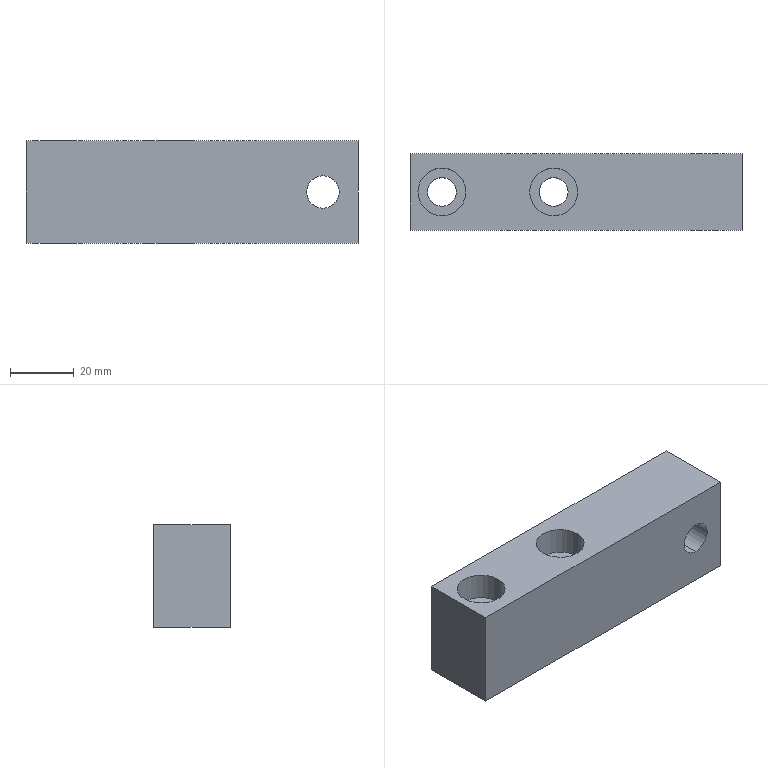Part | STEP file | PN_0036 (positioning fixed block) | 1 solid | 24 faces | box 104 x 24 x 32 mm | volume 69858 mm3 | cylinder 14 | plane 10 | commonest cylinder face diameters 15 x8 9 x4 10.2 x2